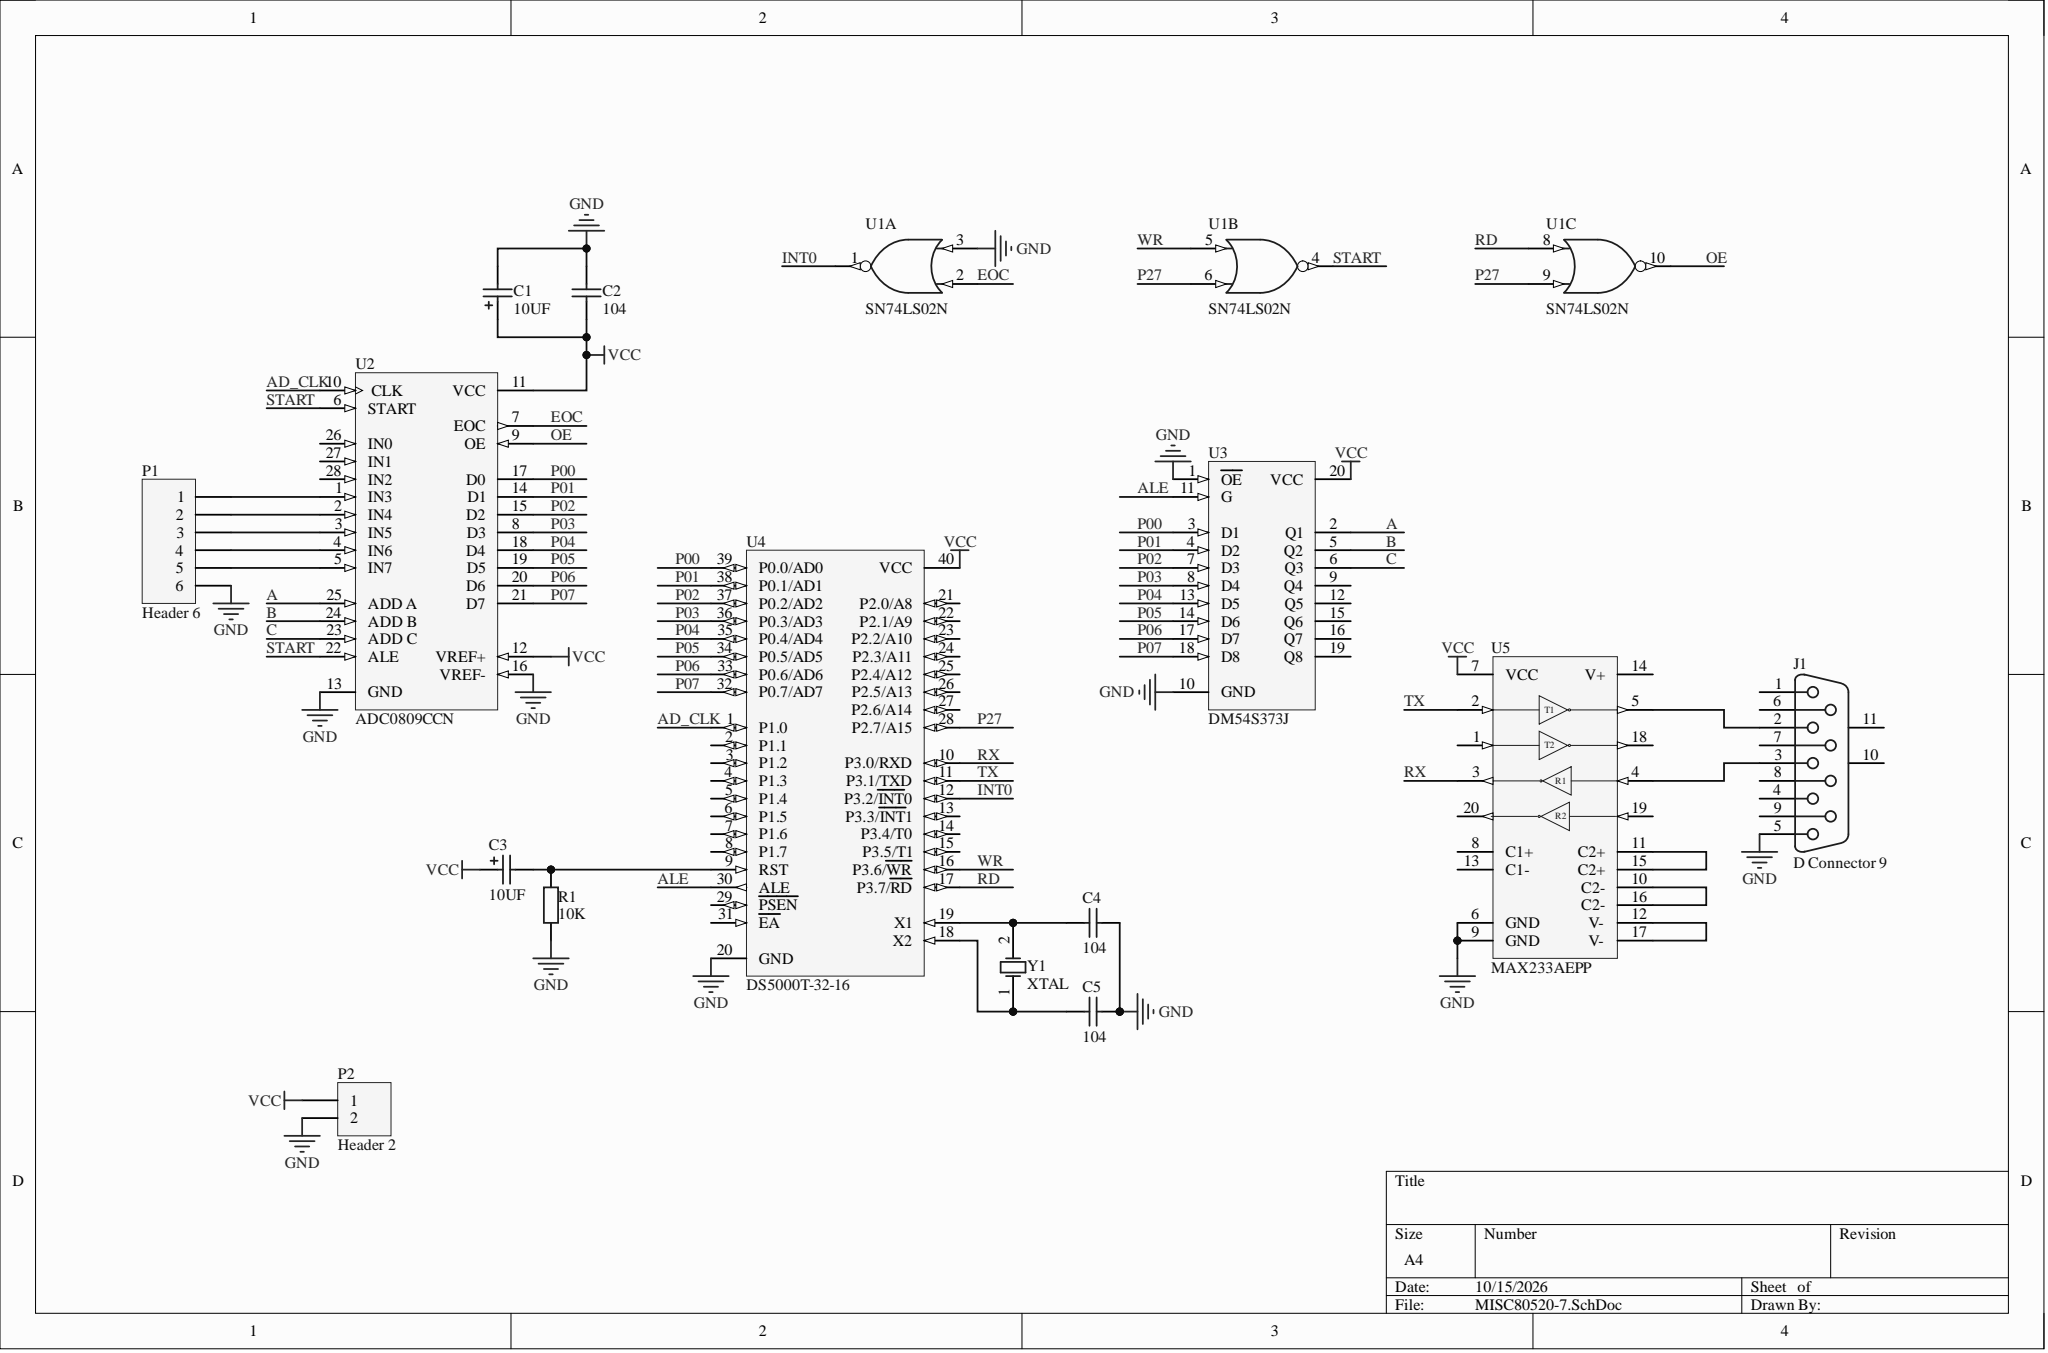Circuit board | Altium Designer | 15 parts | 37 nets
Bill of materials:
Comment,Description,Designator,Footprint,LibRef,Quantity
"10UF","Polarized Capacitor (Axial)","C1, C3","POLAR0.8","Cap Pol2","2"
"104","Capacitor","C2, C4, C5","RAD-0.1","Cap","3"
"D Connector 9","Receptacle Assembly, 9 Position, Right Angle","J1","DSUB1.385-2H9","D Connector 9","1"
"Header 6","Header, 6-Pin","P1","HDR1X6","Header 6","1"
"Header 2","Header, 2-Pin","P2","HDR1X2","Header 2","1"
"10K","Resistor","R1","AXIAL-0.4","Res2","1"
"SN74LS02N","Quadruple 2-Input Positive-NOR Gate","U1","N014","SN74LS02N","1"
"ADC0809CCN","8-Bit µP-Compatible A/D Converter with 8-Channel Multiplexer","U2","N28B","ADC0809CCN","1"
"DM54S373J","Octal D-Type Transparent Latch and Edge-Triggered Flip-Flop","U3","J20A","DM54S373J","1"
"DS5000T-32-16","Soft Microcontroller","U4","ENDIP40A","DS5000T-32-16","1"
"MAX233AEPP","+5V-Powered, Multichannel RS-232 Driver/Receiver","U5","PP20","MAX233AEPP","1"
"XTAL","Crystal Oscillator","Y1","R38","XTAL","1"
Netlist (Protel format):
[
C1
POLAR0.8
10UF



]
[
C2
RAD-0.1
104



]
[
C3
POLAR0.8
10UF



]
[
C4
RAD-0.1
104



]
[
C5
RAD-0.1
104



]
[
J1
DSUB1.385-2H9
D Connector 9



]
[
P1
HDR1X6
Header 6



]
[
P2
HDR1X2
Header 2



]
[
R1
AXIAL-0.4
10K



]
[
U1
N014
SN74LS02N



]
[
U2
N28B
ADC0809CCN



]
[
U3
J20A
DM54S373J



]
[
U4
ENDIP40A
DS5000T-32-16



]
[
U5
PP20
MAX233AEPP



]
[
Y1
R38
XTAL



]
(
WR
U1-5
U4-16
)
(
VCC
C1-1
C2-1
C3-1
P2-1
U1-14
U2-11
U2-12
U3-20
U4-40
U5-7
)
(
TX
U4-11
U5-2
)
(
START
U1-4
U2-6
U2-22
)
(
RX
U4-10
U5-3
)
(
RD
U1-8
U4-17
)
(
P27
U1-6
U1-9
U4-28
)
(
P07
U2-21
U3-18
U4-32
)
(
P06
U2-20
U3-17
U4-33
)
(
P05
U2-19
U3-14
U4-34
)
(
P04
U2-18
U3-13
U4-35
)
(
P03
U2-8
U3-8
U4-36
)
(
P02
U2-15
U3-7
U4-37
)
(
P01
U2-14
U3-4
U4-38
)
(
P00
U2-17
U3-3
U4-39
)
(
OE
U1-10
U2-9
)
(
NetU5_12
U5-12
U5-17
)
(
NetU5_11
U5-11
U5-15
)
(
NetU5_10
U5-10
U5-16
)
(
NetP1_5
P1-5
U2-5
)
(
NetP1_4
P1-4
U2-4
)
(
NetP1_3
P1-3
U2-3
)
(
NetP1_2
P1-2
U2-2
)
(
NetP1_1
P1-1
U2-1
)
(
NetJ1_3
J1-3
U5-4
)
(
NetJ1_2
J1-2
U5-5
)
(
NetC5_1
C5-1
U4-18
Y1-1
)
(
NetC4_2
C4-2
U4-19
Y1-2
)
(
NetC3_2
C3-2
R1-2
U4-9
)
(
INT0
U1-1
U4-12
)
(
GND
C1-2
C2-2
C4-1
C5-2
J1-5
P1-6
P2-2
R1-1
U1-3
U1-7
U2-13
U2-16
U3-1
U3-10
U4-20
U5-6
U5-9
)
(
EOC
U1-2
U2-7
)
(
C
U2-23
U3-6
)
(
B
U2-24
U3-5
)
(
ALE
U3-11
U4-30
)
(
AD_CLK
U2-10
U4-1
)
(
A
U2-25
U3-2
)